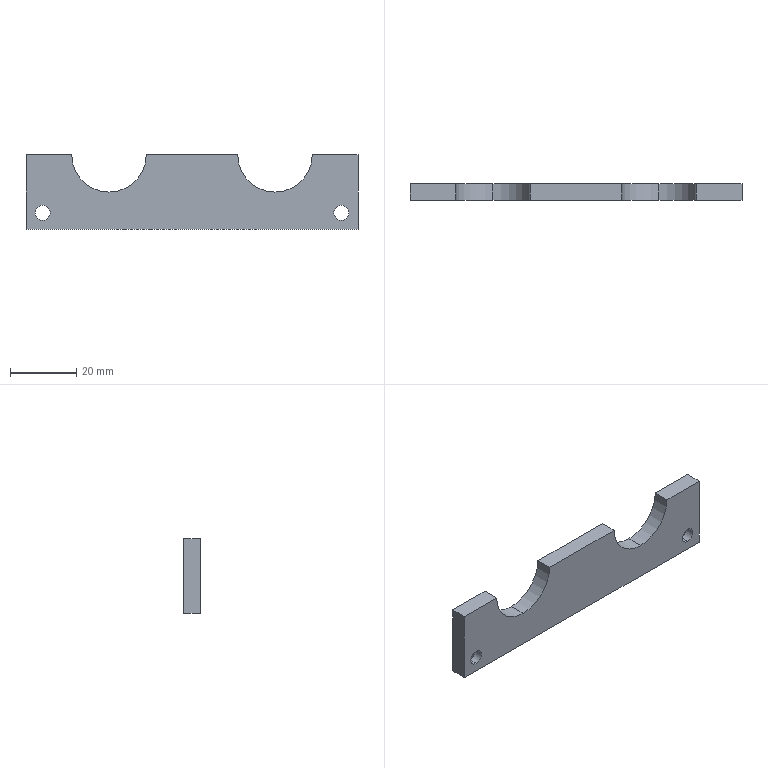Part | STEP file | Ctrl box POM plate | 1 solid | 20 faces | box 100 x 5 x 22.5 mm | volume 9009 mm3 | cylinder 8 | plane 8 | cone 4 | commonest cylinder face diameters 4.5 x4 22.5 x4